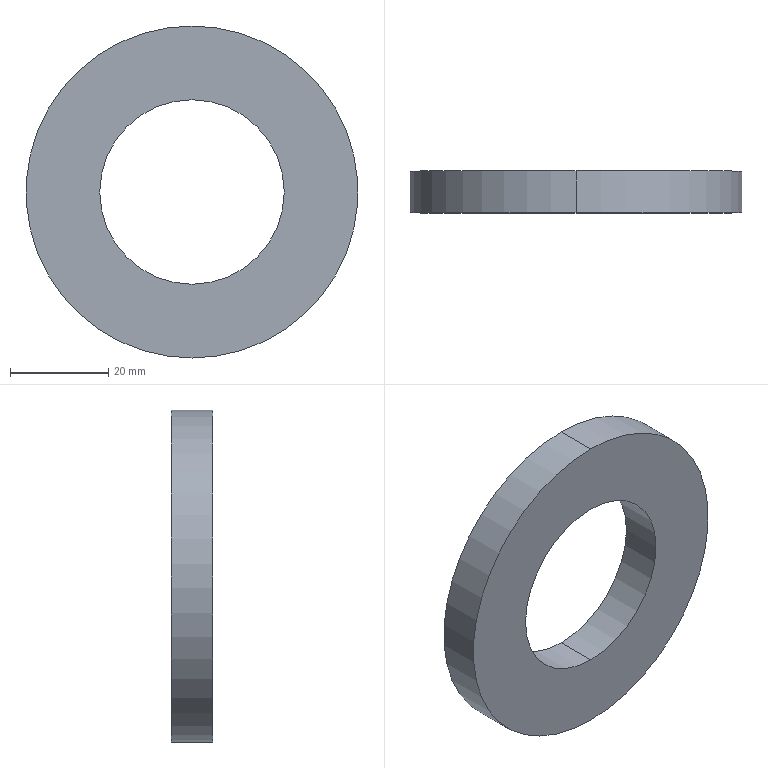Part | STEP file | 2026.6.15-Main Assembly图.sldasm-Part-139 | 1 solid | 6 faces | box 67.5 x 8.5 x 67.5 mm | volume 21029 mm3 | cylinder 4 | plane 2 | commonest cylinder face diameters 37.5 x2 67.5 x2
STEP:
#1=CARTESIAN_POINT('',(-1589.224,534.301,4227.417));
#2=VERTEX_POINT('',#1);
#3=CARTESIAN_POINT('',(-1589.224,534.301,4189.917));
#4=VERTEX_POINT('',#3);
#5=CARTESIAN_POINT('',(-1589.224,534.301,4208.667));
#6=DIRECTION('',(0.,-1.,0.));
#7=DIRECTION('',(0.,0.,-1.));
#8=AXIS2_PLACEMENT_3D('',#5,#6,#7);
#9=CIRCLE('',#8,18.75);
#10=EDGE_CURVE('',#2,#4,#9,.T.);
#11=ORIENTED_EDGE('',*,*,#10,.F.);
#12=CARTESIAN_POINT('',(-1589.224,525.801,4227.417));
#13=VERTEX_POINT('',#12);
#14=CARTESIAN_POINT('',(-1589.224,534.301,4227.417));
#15=DIRECTION('',(0.,-1.,0.));
#16=VECTOR('',#15,1000.);
#17=LINE('',#14,#16);
#18=EDGE_CURVE('',#2,#13,#17,.T.);
#19=ORIENTED_EDGE('',*,*,#18,.T.);
#20=CARTESIAN_POINT('',(-1589.224,525.801,4189.917));
#21=VERTEX_POINT('',#20);
#22=CARTESIAN_POINT('',(-1589.224,525.801,4208.667));
#23=DIRECTION('',(0.,-1.,0.));
#24=DIRECTION('',(0.,0.,-1.));
#25=AXIS2_PLACEMENT_3D('',#22,#23,#24);
#26=CIRCLE('',#25,18.75);
#27=EDGE_CURVE('',#13,#21,#26,.T.);
#28=ORIENTED_EDGE('',*,*,#27,.T.);
#29=CARTESIAN_POINT('',(-1589.224,534.301,4189.917));
#30=DIRECTION('',(0.,-1.,0.));
#31=VECTOR('',#30,1000.);
#32=LINE('',#29,#31);
#33=EDGE_CURVE('',#4,#21,#32,.T.);
#34=ORIENTED_EDGE('',*,*,#33,.F.);
#35=EDGE_LOOP('',(#11,#19,#28,#34));
#36=FACE_OUTER_BOUND('',#35,.T.);
#37=CARTESIAN_POINT('',(-1589.224,534.301,4208.667));
#38=DIRECTION('',(0.,-1.,0.));
#39=DIRECTION('',(0.,0.,-1.));
#40=AXIS2_PLACEMENT_3D('',#37,#38,#39);
#41=CYLINDRICAL_SURFACE('',#40,18.75);
#42=ADVANCED_FACE('',(#36),#41,.F.);
#43=CARTESIAN_POINT('',(-1589.224,525.801,4242.417));
#44=VERTEX_POINT('',#43);
#45=CARTESIAN_POINT('',(-1589.224,525.801,4174.917));
#46=VERTEX_POINT('',#45);
#47=CARTESIAN_POINT('',(-1589.224,525.801,4208.667));
#48=DIRECTION('',(0.,1.,0.));
#49=DIRECTION('',(0.,0.,1.));
#50=AXIS2_PLACEMENT_3D('',#47,#48,#49);
#51=CIRCLE('',#50,33.75);
#52=EDGE_CURVE('',#44,#46,#51,.T.);
#53=ORIENTED_EDGE('',*,*,#52,.T.);
#54=CARTESIAN_POINT('',(-1589.224,534.301,4174.917));
#55=VERTEX_POINT('',#54);
#56=CARTESIAN_POINT('',(-1589.224,525.801,4174.917));
#57=DIRECTION('',(0.,1.,0.));
#58=VECTOR('',#57,1000.);
#59=LINE('',#56,#58);
#60=EDGE_CURVE('',#46,#55,#59,.T.);
#61=ORIENTED_EDGE('',*,*,#60,.T.);
#62=CARTESIAN_POINT('',(-1589.224,534.301,4242.417));
#63=VERTEX_POINT('',#62);
#64=CARTESIAN_POINT('',(-1589.224,534.301,4208.667));
#65=DIRECTION('',(0.,-1.,0.));
#66=DIRECTION('',(0.,0.,1.));
#67=AXIS2_PLACEMENT_3D('',#64,#65,#66);
#68=CIRCLE('',#67,33.75);
#69=EDGE_CURVE('',#55,#63,#68,.T.);
#70=ORIENTED_EDGE('',*,*,#69,.T.);
#71=CARTESIAN_POINT('',(-1589.224,525.801,4242.417));
#72=DIRECTION('',(0.,1.,0.));
#73=VECTOR('',#72,1000.);
#74=LINE('',#71,#73);
#75=EDGE_CURVE('',#44,#63,#74,.T.);
#76=ORIENTED_EDGE('',*,*,#75,.F.);
#77=EDGE_LOOP('',(#53,#61,#70,#76));
#78=FACE_OUTER_BOUND('',#77,.T.);
#79=CARTESIAN_POINT('',(-1589.224,525.801,4208.667));
#80=DIRECTION('',(0.,1.,0.));
#81=DIRECTION('',(0.,0.,1.));
#82=AXIS2_PLACEMENT_3D('',#79,#80,#81);
#83=CYLINDRICAL_SURFACE('',#82,33.75);
#84=ADVANCED_FACE('',(#78),#83,.T.);
#85=CARTESIAN_POINT('',(-1589.224,534.301,4208.667));
#86=DIRECTION('',(0.,-1.,0.));
#87=DIRECTION('',(0.,0.,-1.));
#88=AXIS2_PLACEMENT_3D('',#85,#86,#87);
#89=CIRCLE('',#88,18.75);
#90=EDGE_CURVE('',#4,#2,#89,.T.);
#91=ORIENTED_EDGE('',*,*,#90,.T.);
#92=ORIENTED_EDGE('',*,*,#10,.T.);
#93=EDGE_LOOP('',(#91,#92));
#94=FACE_BOUND('',#93,.T.);
#95=CARTESIAN_POINT('',(-1589.224,534.301,4208.667));
#96=DIRECTION('',(0.,-1.,0.));
#97=DIRECTION('',(0.,0.,1.));
#98=AXIS2_PLACEMENT_3D('',#95,#96,#97);
#99=CIRCLE('',#98,33.75);
#100=EDGE_CURVE('',#63,#55,#99,.T.);
#101=ORIENTED_EDGE('',*,*,#100,.F.);
#102=ORIENTED_EDGE('',*,*,#69,.F.);
#103=EDGE_LOOP('',(#101,#102));
#104=FACE_OUTER_BOUND('',#103,.T.);
#105=CARTESIAN_POINT('',(-1589.224,534.301,4208.667));
#106=DIRECTION('',(0.,1.,0.));
#107=DIRECTION('',(0.,0.,1.));
#108=AXIS2_PLACEMENT_3D('',#105,#106,#107);
#109=PLANE('',#108);
#110=ADVANCED_FACE('',(#94,#104),#109,.T.);
#111=CARTESIAN_POINT('',(-1589.224,525.801,4208.667));
#112=DIRECTION('',(0.,-1.,0.));
#113=DIRECTION('',(0.,0.,-1.));
#114=AXIS2_PLACEMENT_3D('',#111,#112,#113);
#115=CIRCLE('',#114,18.75);
#116=EDGE_CURVE('',#21,#13,#115,.T.);
#117=ORIENTED_EDGE('',*,*,#116,.F.);
#118=ORIENTED_EDGE('',*,*,#27,.F.);
#119=EDGE_LOOP('',(#117,#118));
#120=FACE_BOUND('',#119,.T.);
#121=ORIENTED_EDGE('',*,*,#52,.F.);
#122=CARTESIAN_POINT('',(-1589.224,525.801,4208.667));
#123=DIRECTION('',(0.,1.,0.));
#124=DIRECTION('',(0.,0.,1.));
#125=AXIS2_PLACEMENT_3D('',#122,#123,#124);
#126=CIRCLE('',#125,33.75);
#127=EDGE_CURVE('',#46,#44,#126,.T.);
#128=ORIENTED_EDGE('',*,*,#127,.F.);
#129=EDGE_LOOP('',(#121,#128));
#130=FACE_OUTER_BOUND('',#129,.T.);
#131=CARTESIAN_POINT('',(-1589.224,525.801,4208.667));
#132=DIRECTION('',(0.,-1.,0.));
#133=DIRECTION('',(0.,0.,-1.));
#134=AXIS2_PLACEMENT_3D('',#131,#132,#133);
#135=PLANE('',#134);
#136=ADVANCED_FACE('',(#120,#130),#135,.T.);
#137=ORIENTED_EDGE('',*,*,#60,.F.);
#138=ORIENTED_EDGE('',*,*,#127,.T.);
#139=ORIENTED_EDGE('',*,*,#75,.T.);
#140=ORIENTED_EDGE('',*,*,#100,.T.);
#141=EDGE_LOOP('',(#137,#138,#139,#140));
#142=FACE_OUTER_BOUND('',#141,.T.);
#143=CARTESIAN_POINT('',(-1589.224,525.801,4208.667));
#144=DIRECTION('',(0.,1.,0.));
#145=DIRECTION('',(0.,0.,1.));
#146=AXIS2_PLACEMENT_3D('',#143,#144,#145);
#147=CYLINDRICAL_SURFACE('',#146,33.75);
#148=ADVANCED_FACE('',(#142),#147,.T.);
#149=ORIENTED_EDGE('',*,*,#18,.F.);
#150=ORIENTED_EDGE('',*,*,#90,.F.);
#151=ORIENTED_EDGE('',*,*,#33,.T.);
#152=ORIENTED_EDGE('',*,*,#116,.T.);
#153=EDGE_LOOP('',(#149,#150,#151,#152));
#154=FACE_OUTER_BOUND('',#153,.T.);
#155=CARTESIAN_POINT('',(-1589.224,534.301,4208.667));
#156=DIRECTION('',(0.,-1.,0.));
#157=DIRECTION('',(0.,0.,-1.));
#158=AXIS2_PLACEMENT_3D('',#155,#156,#157);
#159=CYLINDRICAL_SURFACE('',#158,18.75);
#160=ADVANCED_FACE('',(#154),#159,.F.);
#161=CLOSED_SHELL('',(#42,#84,#110,#136,#148,#160));
#162=MANIFOLD_SOLID_BREP('',#161);
#163=CARTESIAN_POINT('',(0.,0.,0.));
#164=DIRECTION('',(0.,0.,1.));
#165=DIRECTION('',(1.,0.,0.));
#166=AXIS2_PLACEMENT_3D('',#163,#164,#165);
#167=(LENGTH_UNIT()NAMED_UNIT(*)SI_UNIT(.MILLI.,.METRE.));
#168=UNCERTAINTY_MEASURE_WITH_UNIT(LENGTH_MEASURE(0.00001),#167,'','');
#169=(NAMED_UNIT(*)PLANE_ANGLE_UNIT()SI_UNIT($,.RADIAN.));
#170=(NAMED_UNIT(*)SI_UNIT($,.STERADIAN.)SOLID_ANGLE_UNIT());
#171=(GEOMETRIC_REPRESENTATION_CONTEXT(3)GLOBAL_UNCERTAINTY_ASSIGNED_CONTEXT((#168))GLOBAL_UNIT_ASSIGNED_CONTEXT((#167,#169,#170))REPRESENTATION_CONTEXT('',''));
#172=ADVANCED_BREP_SHAPE_REPRESENTATION('',(#162,#166),#171);